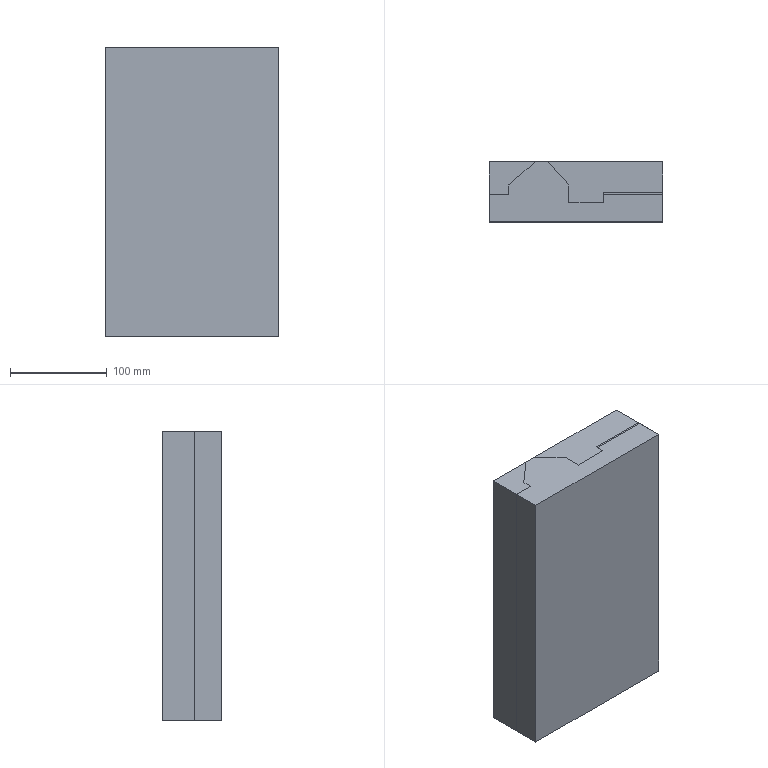NC program | NX | posted with a generic post | part box 180 x 62 x 300 mm
Lines 29267 to 29776 of 29776:
(等高外形 , TOOL : D21R0.8圆鼻飞刀)
N58520 T04 M6
N58522 /M1
N58524 G54
N58526 G17 G0 G90 X172.5 Y-82. S1500 M3
N58528 G43 Z20. H4
N58530 Z-24.682
N58532 G94 G1 Z-24.882 F1600.
N58534 X150.
N58536 X-150. F2000.
N58538 X-172.5
N58540 G0 Z-23.8
N58542 Z-24.976
N58544 G1 Z-25.176 F1600.
N58546 X-150.
N58548 X150. F2000.
N58550 X172.5
N58552 G0 Z-24.682
N58554 Z-25.271
N58556 G1 Z-25.471 F1600.
N58558 X150.
N58560 X-150. F2000.
N58562 X-172.5
N58564 G0 Z-24.976
N58566 Z-25.565
N58568 G1 Z-25.765 F1600.
N58570 X-150.
N58572 X150. F2000.
N58574 X172.5
N58576 G0 Z-25.271
N58578 Z-25.859
N58580 G1 Z-26.059 F1600.
N58582 X150.
N58584 X-150. F2000.
N58586 X-172.5
N58588 G0 Z-25.565
N58590 Z-26.153
N58592 G1 Z-26.353 F1600.
N58594 X-150.
N58596 X150. F2000.
N58598 X172.5
N58600 G0 Z-25.859
N58602 Z-26.447
N58604 G1 Z-26.647 F1600.
N58606 X150.
N58608 X-150. F2000.
N58610 X-172.5
N58612 G0 Z-26.153
N58614 Z-26.741
N58616 G1 Z-26.941 F1600.
N58618 X-150.
N58620 X150. F2000.
N58622 X172.5
N58624 G0 Z-26.447
N58626 Z-27.035
N58628 G1 Z-27.235 F1600.
N58630 X150.
N58632 X-150. F2000.
N58634 X-172.5
N58636 G0 Z-26.741
N58638 Z-27.329
N58640 G1 Z-27.529 F1600.
N58642 X-150.
N58644 X150. F2000.
N58646 X172.5
N58648 G0 Z-27.035
N58650 Z-27.624
N58652 G1 Z-27.824 F1600.
N58654 X150.
N58656 X-150. F2000.
N58658 X-172.5
N58660 G0 Z-27.329
N58662 Z-27.918
N58664 G1 Z-28.118 F1600.
N58666 X-150.
N58668 X150. F2000.
N58670 X172.5
N58672 G0 Z-27.624
N58674 Z-28.212
N58676 G1 Z-28.412 F1600.
N58678 X150.
N58680 X-150. F2000.
N58682 X-172.5
N58684 G0 Z-27.918
N58686 Z-28.506
N58688 G1 Z-28.706 F1600.
N58690 X-150.
N58692 X150. F2000.
N58694 X172.5
N58696 G0 Z-28.212
N58698 Z-28.8
N58700 G1 Z-29. F1600.
N58702 X150.
N58704 X-150. F2000.
N58706 X-172.5
N58708 G0 Z-28.506
N58710 Z-29.094
N58712 G1 Z-29.294 F1600.
N58714 X-150.
N58716 X150. F2000.
N58718 X172.5
N58720 G0 Z-28.8
N58722 Z-29.388
N58724 G1 Z-29.588 F1600.
N58726 X150.
N58728 X-150. F2000.
N58730 X-172.5
N58732 G0 Z-29.094
N58734 Z-29.682
N58736 G1 Z-29.882 F1600.
N58738 X-150.
N58740 X150. F2000.
N58742 X172.5
N58744 G0 Z-29.388
N58746 Z-29.976
N58748 G1 Z-30.176 F1600.
N58750 X150.
N58752 X-150. F2000.
N58754 X-172.5
N58756 G0 Z-29.682
N58758 Z-30.271
N58760 G1 Z-30.471 F1600.
N58762 X-150.
N58764 X150. F2000.
N58766 X172.5
N58768 G0 Z-29.976
N58770 Z-30.565
N58772 G1 Z-30.765 F1600.
N58774 X150.
N58776 X-150. F2000.
N58778 X-172.5
N58780 G0 Z-30.271
N58782 Z-30.859
N58784 G1 Z-31.059 F1600.
N58786 X-150.
N58788 X150. F2000.
N58790 X172.5
N58792 G0 Z-30.565
N58794 Z-31.153
N58796 G1 Z-31.353 F1600.
N58798 X150.
N58800 X-150. F2000.
N58802 X-172.5
N58804 G0 Z-30.859
N58806 Z-31.447
N58808 G1 Z-31.647 F1600.
N58810 X-150.
N58812 X150. F2000.
N58814 X172.5
N58816 G0 Z-31.153
N58818 Z-31.741
N58820 G1 Z-31.941 F1600.
N58822 X150.
N58824 X-150. F2000.
N58826 X-172.5
N58828 G0 Z-31.447
N58830 Z-32.035
N58832 G1 Z-32.235 F1600.
N58834 X-150.
N58836 X150. F2000.
N58838 X172.5
N58840 G0 Z-31.741
N58842 Z-32.329
N58844 G1 Z-32.529 F1600.
N58846 X150.
N58848 X-150. F2000.
N58850 X-172.5
N58852 G0 Z-32.035
N58854 Z-32.624
N58856 G1 Z-32.824 F1600.
N58858 X-150.
N58860 X150. F2000.
N58862 X172.5
N58864 G0 Z-32.329
N58866 Z-32.918
N58868 G1 Z-33.118 F1600.
N58870 X150.
N58872 X-150. F2000.
N58874 X-172.5
N58876 G0 Z-32.624
N58878 Z-33.212
N58880 G1 Z-33.412 F1600.
N58882 X-150.
N58884 X150. F2000.
N58886 X172.5
N58888 G0 Z-32.918
N58890 Z-33.506
N58892 G1 Z-33.706 F1600.
N58894 X150.
N58896 X-150. F2000.
N58898 X-172.5
N58900 G0 Z-33.212
N58902 Z-33.8
N58904 G1 Z-34. F1600.
N58906 X-150.
N58908 X150. F2000.
N58910 X172.5
N58912 G0 Z20.
(飞平面_1 , TOOL : D21R0.8圆鼻飞刀)
N58914 /M1
N58916 X-164.998 Y15.998
N58918 Z-33.796
N58920 G1 Z-34.296 F1600.
N58922 X-149.998
N58924 X157.998 F2000.
N58926 G2 X162.498 Y11.498 R4.5
N58928 G1 Y10.
N58930 G2 X157.498 Y5. R5.
N58932 G1 X-162.498
N58934 G0 Z-33.5
N58936 X-164.998 Y15.998
N58938 Z-34.093
N58940 G1 Z-34.593 F1600.
N58942 X-149.998
N58944 X157.998 F2000.
N58946 G2 X162.498 Y11.498 R4.5
N58948 G1 Y10.
N58950 G2 X157.498 Y5. R5.
N58952 G1 X-162.498
N58954 G0 Z-33.796
N58956 X-164.998 Y15.998
N58958 Z-34.389
N58960 G1 Z-34.889 F1600.
N58962 X-149.998
N58964 X157.998 F2000.
N58966 G2 X162.498 Y11.498 R4.5
N58968 G1 Y10.
N58970 G2 X157.498 Y5. R5.
N58972 G1 X-162.498
N58974 G0 Z-34.093
N58976 X-164.998 Y15.998
N58978 Z-34.685
N58980 G1 Z-35.185 F1600.
N58982 X-149.998
N58984 X157.998 F2000.
N58986 G2 X162.498 Y11.498 R4.5
N58988 G1 Y10.
N58990 G2 X157.498 Y5. R5.
N58992 G1 X-162.498
N58994 G0 Z-34.389
N58996 X-164.998 Y15.998
N58998 Z-34.981
N59000 G1 Z-35.481 F1600.
N59002 X-149.998
N59004 X157.998 F2000.
N59006 G2 X162.498 Y11.498 R4.5
N59008 G1 Y10.
N59010 G2 X157.498 Y5. R5.
N59012 G1 X-162.498
N59014 G0 Z-34.685
N59016 X-164.998 Y15.998
N59018 Z-35.278
N59020 G1 Z-35.778 F1600.
N59022 X-149.998
N59024 X157.998 F2000.
N59026 G2 X162.498 Y11.498 R4.5
N59028 G1 Y10.
N59030 G2 X157.498 Y5. R5.
N59032 G1 X-162.498
N59034 G0 Z-34.981
N59036 X-164.998 Y15.998
N59038 Z-35.574
N59040 G1 Z-36.074 F1600.
N59042 X-149.998
N59044 X157.998 F2000.
N59046 G2 X162.498 Y11.498 R4.5
N59048 G1 Y10.
N59050 G2 X157.498 Y5. R5.
N59052 G1 X-162.498
N59054 G0 Z-35.278
N59056 X-164.998 Y15.998
N59058 Z-35.87
N59060 G1 Z-36.37 F1600.
N59062 X-149.998
N59064 X157.998 F2000.
N59066 G2 X162.498 Y11.498 R4.5
N59068 G1 Y10.
N59070 G2 X157.498 Y5. R5.
N59072 G1 X-162.498
N59074 G0 Z-35.574
N59076 X-164.998 Y15.998
N59078 Z-36.167
N59080 G1 Z-36.667 F1600.
N59082 X-149.998
N59084 X157.998 F2000.
N59086 G2 X162.498 Y11.498 R4.5
N59088 G1 Y10.
N59090 G2 X157.498 Y5. R5.
N59092 G1 X-162.498
N59094 G0 Z-35.87
N59096 X-164.998 Y15.998
N59098 Z-36.463
N59100 G1 Z-36.963 F1600.
N59102 X-149.998
N59104 X157.998 F2000.
N59106 G2 X162.498 Y11.498 R4.5
N59108 G1 Y10.
N59110 G2 X157.498 Y5. R5.
N59112 G1 X-162.498
N59114 G0 Z-36.167
N59116 X-164.998 Y15.998
N59118 Z-36.759
N59120 G1 Z-37.259 F1600.
N59122 X-149.998
N59124 X157.998 F2000.
N59126 G2 X162.498 Y11.498 R4.5
N59128 G1 Y10.
N59130 G2 X157.498 Y5. R5.
N59132 G1 X-162.498
N59134 G0 Z-36.463
N59136 X-164.998 Y15.998
N59138 Z-37.056
N59140 G1 Z-37.556 F1600.
N59142 X-149.998
N59144 X157.998 F2000.
N59146 G2 X162.498 Y11.498 R4.5
N59148 G1 Y10.
N59150 G2 X157.498 Y5. R5.
N59152 G1 X-162.498
N59154 G0 Z-36.759
N59156 X-164.998 Y15.998
N59158 Z-37.352
N59160 G1 Z-37.852 F1600.
N59162 X-149.998
N59164 X157.998 F2000.
N59166 G2 X162.498 Y11.498 R4.5
N59168 G1 Y10.
N59170 G2 X157.498 Y5. R5.
N59172 G1 X-162.498
N59174 G0 Z-37.056
N59176 X-164.998 Y15.998
N59178 Z-37.648
N59180 G1 Z-38.148 F1600.
N59182 X-149.998
N59184 X157.998 F2000.
N59186 G2 X162.498 Y11.498 R4.5
N59188 G1 Y10.
N59190 G2 X157.498 Y5. R5.
N59192 G1 X-162.498
N59194 G0 Z-37.352
N59196 X-164.998 Y15.998
N59198 Z-37.944
N59200 G1 Z-38.444 F1600.
N59202 X-149.998
N59204 X157.998 F2000.
N59206 G2 X162.498 Y11.498 R4.5
N59208 G1 Y10.
N59210 G2 X157.498 Y5. R5.
N59212 G1 X-162.498
N59214 G0 Z-37.648
N59216 X-164.998 Y15.998
N59218 Z-38.241
N59220 G1 Z-38.741 F1600.
N59222 X-149.998
N59224 X157.998 F2000.
N59226 G2 X162.498 Y11.498 R4.5
N59228 G1 Y10.
N59230 G2 X157.498 Y5. R5.
N59232 G1 X-162.498
N59234 G0 Z-37.944
N59236 X-164.998 Y15.998
N59238 Z-38.537
N59240 G1 Z-39.037 F1600.
N59242 X-149.998
N59244 X157.998 F2000.
N59246 G2 X162.498 Y11.498 R4.5
N59248 G1 Y10.
N59250 G2 X157.498 Y5. R5.
N59252 G1 X-162.498
N59254 G0 Z-38.241
N59256 X-164.998 Y15.998
N59258 Z-38.833
N59260 G1 Z-39.333 F1600.
N59262 X-149.998
N59264 X157.998 F2000.
N59266 G2 X162.498 Y11.498 R4.5
N59268 G1 Y10.
N59270 G2 X157.498 Y5. R5.
N59272 G1 X-162.498
N59274 G0 Z-38.537
N59276 X-164.998 Y15.998
N59278 Z-39.13
N59280 G1 Z-39.63 F1600.
N59282 X-149.998
N59284 X157.998 F2000.
N59286 G2 X162.498 Y11.498 R4.5
N59288 G1 Y10.
N59290 G2 X157.498 Y5. R5.
N59292 G1 X-162.498
N59294 G0 Z-38.833
N59296 X-164.998 Y15.998
N59298 Z-39.426
N59300 G1 Z-39.926 F1600.
N59302 X-149.998
N59304 X157.998 F2000.
N59306 G2 X162.498 Y11.498 R4.5
N59308 G1 Y10.
N59310 G2 X157.498 Y5. R5.
N59312 G1 X-162.498
N59314 G0 Z-39.13
N59316 X-164.998 Y15.998
N59318 Z-39.722
N59320 G1 Z-40.222 F1600.
N59322 X-149.998
N59324 X157.998 F2000.
N59326 G2 X162.498 Y11.498 R4.5
N59328 G1 Y10.
N59330 G2 X157.498 Y5. R5.
N59332 G1 X-162.498
N59334 G0 Z-39.426
N59336 X-164.998 Y15.998
N59338 Z-40.019
N59340 G1 Z-40.519 F1600.
N59342 X-149.998
N59344 X157.998 F2000.
N59346 G2 X162.498 Y11.498 R4.5
N59348 G1 Y10.
N59350 G2 X157.498 Y5. R5.
N59352 G1 X-162.498
N59354 G0 Z-39.722
N59356 X-164.998 Y15.998
N59358 Z-40.315
N59360 G1 Z-40.815 F1600.
N59362 X-149.998
N59364 X157.998 F2000.
N59366 G2 X162.498 Y11.498 R4.5
N59368 G1 Y10.
N59370 G2 X157.498 Y5. R5.
N59372 G1 X-162.498
N59374 G0 Z-40.019
N59376 X-164.998 Y15.998
N59378 Z-40.611
N59380 G1 Z-41.111 F1600.
N59382 X-149.998
N59384 X157.998 F2000.
N59386 G2 X162.498 Y11.498 R4.5
N59388 G1 Y10.
N59390 G2 X157.498 Y5. R5.
N59392 G1 X-162.498
N59394 G0 Z-40.315
N59396 X-164.998 Y15.998
N59398 Z-40.907
N59400 G1 Z-41.407 F1600.
N59402 X-149.998
N59404 X157.998 F2000.
N59406 G2 X162.498 Y11.498 R4.5
N59408 G1 Y10.
N59410 G2 X157.498 Y5. R5.
N59412 G1 X-162.498
N59414 G0 Z-40.611
N59416 X-164.998 Y15.998
N59418 Z-41.204
N59420 G1 Z-41.704 F1600.
N59422 X-149.998
N59424 X157.998 F2000.
N59426 G2 X162.498 Y11.498 R4.5
N59428 G1 Y10.
N59430 G2 X157.498 Y5. R5.
N59432 G1 X-162.498
N59434 G0 Z-40.907
N59436 X-164.998 Y15.998
N59438 Z-41.5
N59440 G1 Z-42. F1600.
N59442 X-149.998
N59444 X157.998 F2000.
N59446 G2 X162.498 Y11.498 R4.5
N59448 G1 Y10.
N59450 G2 X157.498 Y5. R5.
N59452 G1 X-162.498
N59454 G0 Z20.
(飞平面 , TOOL : D21R0.8圆鼻飞刀)
N59456 /M1
N59458 X-184.998 Y101.438 S3000
N59460 Z-33.5
N59462 G1 Z-34. F1200.
N59464 X-169.998
N59466 X177.501 F1500.
N59468 G2 X182.498 Y96.441 R5.
N59470 G1 Y87.328
N59472 G2 X177.498 Y82.328 R5.
N59474 G1 X-177.501
N59476 G3 X-182.498 Y77.332 R5.
N59478 G1 Y67.719
N59480 G3 X-177.998 Y63.219 R4.5
N59482 G1 X177.501
N59484 G2 X182.498 Y58.222 R5.
N59486 G1 Y49.11
N59488 G2 X177.498 Y44.11 R5.
N59490 G1 X-177.501
N59492 G3 X-182.498 Y39.113 R5.
N59494 G1 Y29.5
N59496 G3 X-177.998 Y25. R4.5
N59498 G1 X182.498
N59500 G0 Z20.
N59502 X-186.675 Y-116.407
N59504 Z-33.5
N59506 G1 Z-34. F1200.
N59508 X-182.498 Y-102.
N59510 X-182.15 F1500.
N59512 G2 X-178.721 Y-106.564 R3.57
N59514 G1 X-179.948 Y-110.796
N59516 G0 Z20.
N59518 M5
N59520 M2